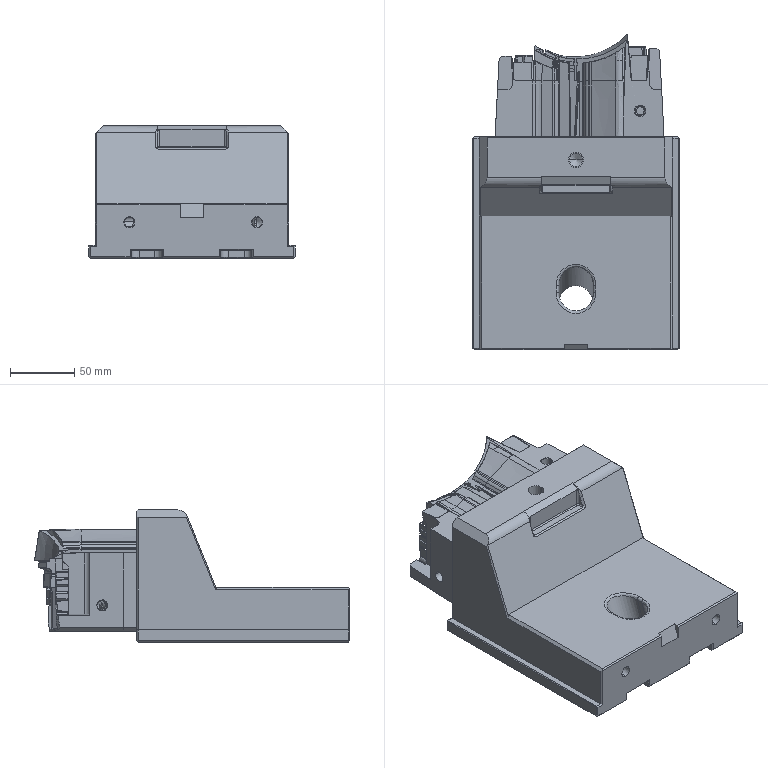Part | Creo | 1 solid | 1048 faces | box 160 x 244.263 x 102.5 mm | volume 1890999 mm3 | plane 367 | cylinder 352 | spline 195 | sphere 62 | cone 46 | other 19 | torus 7 | commonest cylinder face diameters 0.402 x148 2.01 x28 8 x12 1.005 x8 4 x8 8.5 x8